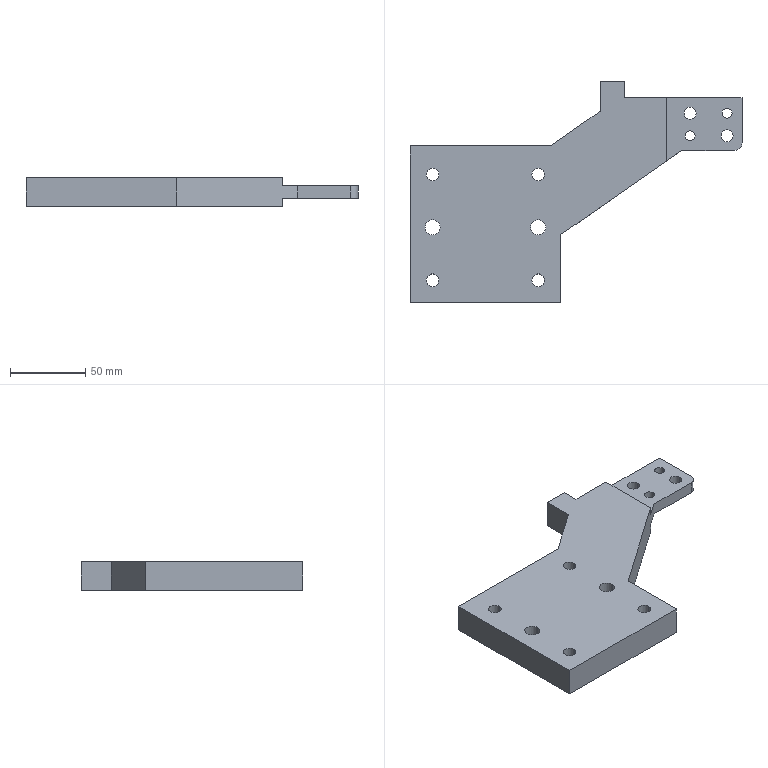Part | SolidWorks | features ICE 4, Extrusion 1, Fillet 1 | 1 solid | 51 faces | box 220 x 147 x 19 mm | volume 284001 mm3 | cylinder 29 | plane 22 | commonest cylinder face diameters 8 x8 8.376 x8 10 x5 6.647 x4 4.917 x2 6.65 x2